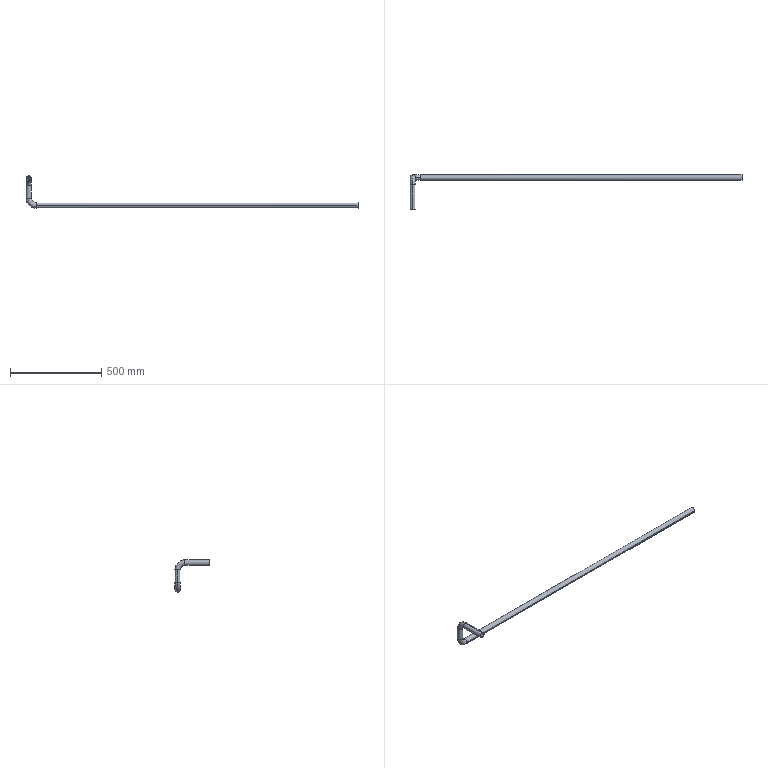Part | SolidWorks | features 3DProfileFeature 2, Sweep 1 | 1 solid | 22 faces | box 1817 x 186.765 x 176.777 mm | volume 367085 mm3 | cylinder 12 | torus 8 | plane 2 | commonest cylinder face diameters 26 x6 30 x6
STEP:
#1=CARTESIAN_POINT('',(-2187.,3372.936,-6.777));
#2=VERTEX_POINT('',#1);
#3=CARTESIAN_POINT('',(-2213.,3372.936,-6.777));
#4=VERTEX_POINT('',#3);
#5=CARTESIAN_POINT('',(-2200.,3372.936,-6.777));
#6=DIRECTION('',(0.,0.,1.));
#7=DIRECTION('',(-1.,0.,0.));
#8=AXIS2_PLACEMENT_3D('',#5,#6,#7);
#9=CIRCLE('',#8,13.);
#10=EDGE_CURVE('',#2,#4,#9,.T.);
#11=ORIENTED_EDGE('',*,*,#10,.T.);
#12=CARTESIAN_POINT('',(-2160.,3372.936,-59.777));
#13=VERTEX_POINT('',#12);
#14=CARTESIAN_POINT('',(-2160.,3372.936,-6.777));
#15=DIRECTION('',(0.,-1.,0.));
#16=DIRECTION('',(0.,0.,-1.));
#17=AXIS2_PLACEMENT_3D('',#14,#15,#16);
#18=CIRCLE('',#17,53.);
#19=EDGE_CURVE('',#4,#13,#18,.T.);
#20=ORIENTED_EDGE('',*,*,#19,.T.);
#21=CARTESIAN_POINT('',(-2160.,3385.936,-46.777));
#22=VERTEX_POINT('',#21);
#23=CARTESIAN_POINT('',(-2160.,3372.936,-46.777));
#24=DIRECTION('',(-1.,0.,0.));
#25=DIRECTION('',(0.,0.,1.));
#26=AXIS2_PLACEMENT_3D('',#23,#24,#25);
#27=CIRCLE('',#26,13.);
#28=EDGE_CURVE('',#22,#13,#27,.T.);
#29=ORIENTED_EDGE('',*,*,#28,.F.);
#30=CARTESIAN_POINT('',(-2160.,3372.936,-33.777));
#31=VERTEX_POINT('',#30);
#32=CARTESIAN_POINT('',(-2160.,3372.936,-46.777));
#33=DIRECTION('',(-1.,0.,0.));
#34=DIRECTION('',(0.,0.,1.));
#35=AXIS2_PLACEMENT_3D('',#32,#33,#34);
#36=CIRCLE('',#35,13.);
#37=EDGE_CURVE('',#31,#22,#36,.T.);
#38=ORIENTED_EDGE('',*,*,#37,.F.);
#39=CARTESIAN_POINT('',(-2160.,3372.936,-6.777));
#40=DIRECTION('',(0.,-1.,0.));
#41=DIRECTION('',(0.,0.,-1.));
#42=AXIS2_PLACEMENT_3D('',#39,#40,#41);
#43=CIRCLE('',#42,27.);
#44=EDGE_CURVE('',#2,#31,#43,.T.);
#45=ORIENTED_EDGE('',*,*,#44,.F.);
#46=EDGE_LOOP('',(#11,#20,#29,#38,#45));
#47=FACE_OUTER_BOUND('',#46,.T.);
#48=CARTESIAN_POINT('',(-2160.,3372.936,-6.777));
#49=DIRECTION('',(0.,-1.,0.));
#50=DIRECTION('',(0.,0.,-1.));
#51=AXIS2_PLACEMENT_3D('',#48,#49,#50);
#52=TOROIDAL_SURFACE('',#51,40.,13.);
#53=ADVANCED_FACE('',(#47),#52,.F.);
#54=CARTESIAN_POINT('',(-2200.,3332.936,87.));
#55=VERTEX_POINT('',#54);
#56=CARTESIAN_POINT('',(-2200.,3332.936,113.));
#57=VERTEX_POINT('',#56);
#58=CARTESIAN_POINT('',(-2200.,3332.936,100.));
#59=DIRECTION('',(0.,-1.,0.));
#60=DIRECTION('',(0.,0.,1.));
#61=AXIS2_PLACEMENT_3D('',#58,#59,#60);
#62=CIRCLE('',#61,13.);
#63=EDGE_CURVE('',#55,#57,#62,.T.);
#64=ORIENTED_EDGE('',*,*,#63,.T.);
#65=CARTESIAN_POINT('',(-2200.,3385.936,60.));
#66=VERTEX_POINT('',#65);
#67=CARTESIAN_POINT('',(-2200.,3332.936,60.));
#68=DIRECTION('',(-1.,0.,0.));
#69=DIRECTION('',(0.,0.,1.));
#70=AXIS2_PLACEMENT_3D('',#67,#68,#69);
#71=CIRCLE('',#70,53.);
#72=EDGE_CURVE('',#57,#66,#71,.T.);
#73=ORIENTED_EDGE('',*,*,#72,.T.);
#74=CARTESIAN_POINT('',(-2187.,3372.936,60.));
#75=VERTEX_POINT('',#74);
#76=CARTESIAN_POINT('',(-2200.,3372.936,60.));
#77=DIRECTION('',(0.,0.,1.));
#78=DIRECTION('',(0.,-1.,0.));
#79=AXIS2_PLACEMENT_3D('',#76,#77,#78);
#80=CIRCLE('',#79,13.);
#81=EDGE_CURVE('',#75,#66,#80,.T.);
#82=ORIENTED_EDGE('',*,*,#81,.F.);
#83=CARTESIAN_POINT('',(-2200.,3359.936,60.));
#84=VERTEX_POINT('',#83);
#85=CARTESIAN_POINT('',(-2200.,3372.936,60.));
#86=DIRECTION('',(0.,0.,1.));
#87=DIRECTION('',(0.,-1.,0.));
#88=AXIS2_PLACEMENT_3D('',#85,#86,#87);
#89=CIRCLE('',#88,13.);
#90=EDGE_CURVE('',#84,#75,#89,.T.);
#91=ORIENTED_EDGE('',*,*,#90,.F.);
#92=CARTESIAN_POINT('',(-2200.,3332.936,60.));
#93=DIRECTION('',(-1.,0.,0.));
#94=DIRECTION('',(0.,0.,1.));
#95=AXIS2_PLACEMENT_3D('',#92,#93,#94);
#96=CIRCLE('',#95,27.);
#97=EDGE_CURVE('',#55,#84,#96,.T.);
#98=ORIENTED_EDGE('',*,*,#97,.F.);
#99=EDGE_LOOP('',(#64,#73,#82,#91,#98));
#100=FACE_OUTER_BOUND('',#99,.T.);
#101=CARTESIAN_POINT('',(-2200.,3332.936,60.));
#102=DIRECTION('',(-1.,0.,0.));
#103=DIRECTION('',(0.,0.,1.));
#104=AXIS2_PLACEMENT_3D('',#101,#102,#103);
#105=TOROIDAL_SURFACE('',#104,40.,13.);
#106=ADVANCED_FACE('',(#100),#105,.F.);
#107=CARTESIAN_POINT('',(-2215.,3372.936,-6.777));
#108=VERTEX_POINT('',#107);
#109=CARTESIAN_POINT('',(-2185.,3372.936,-6.777));
#110=VERTEX_POINT('',#109);
#111=CARTESIAN_POINT('',(-2200.,3372.936,-6.777));
#112=DIRECTION('',(0.,0.,1.));
#113=DIRECTION('',(0.,-1.,0.));
#114=AXIS2_PLACEMENT_3D('',#111,#112,#113);
#115=CIRCLE('',#114,15.);
#116=EDGE_CURVE('',#108,#110,#115,.T.);
#117=ORIENTED_EDGE('',*,*,#116,.F.);
#118=CARTESIAN_POINT('',(-2160.,3372.936,-61.777));
#119=VERTEX_POINT('',#118);
#120=CARTESIAN_POINT('',(-2160.,3372.936,-6.777));
#121=DIRECTION('',(0.,-1.,0.));
#122=DIRECTION('',(0.,0.,-1.));
#123=AXIS2_PLACEMENT_3D('',#120,#121,#122);
#124=CIRCLE('',#123,55.);
#125=EDGE_CURVE('',#108,#119,#124,.T.);
#126=ORIENTED_EDGE('',*,*,#125,.T.);
#127=CARTESIAN_POINT('',(-2160.,3357.936,-46.777));
#128=VERTEX_POINT('',#127);
#129=CARTESIAN_POINT('',(-2160.,3372.936,-46.777));
#130=DIRECTION('',(-1.,0.,0.));
#131=DIRECTION('',(0.,-1.,0.));
#132=AXIS2_PLACEMENT_3D('',#129,#130,#131);
#133=CIRCLE('',#132,15.);
#134=EDGE_CURVE('',#119,#128,#133,.T.);
#135=ORIENTED_EDGE('',*,*,#134,.T.);
#136=CARTESIAN_POINT('',(-2160.,3372.936,-31.777));
#137=VERTEX_POINT('',#136);
#138=CARTESIAN_POINT('',(-2160.,3372.936,-46.777));
#139=DIRECTION('',(-1.,0.,0.));
#140=DIRECTION('',(0.,-1.,0.));
#141=AXIS2_PLACEMENT_3D('',#138,#139,#140);
#142=CIRCLE('',#141,15.);
#143=EDGE_CURVE('',#128,#137,#142,.T.);
#144=ORIENTED_EDGE('',*,*,#143,.T.);
#145=CARTESIAN_POINT('',(-2160.,3372.936,-6.777));
#146=DIRECTION('',(0.,-1.,0.));
#147=DIRECTION('',(0.,0.,-1.));
#148=AXIS2_PLACEMENT_3D('',#145,#146,#147);
#149=CIRCLE('',#148,25.);
#150=EDGE_CURVE('',#110,#137,#149,.T.);
#151=ORIENTED_EDGE('',*,*,#150,.F.);
#152=EDGE_LOOP('',(#117,#126,#135,#144,#151));
#153=FACE_OUTER_BOUND('',#152,.T.);
#154=CARTESIAN_POINT('',(-2160.,3372.936,-6.777));
#155=DIRECTION('',(0.,-1.,0.));
#156=DIRECTION('',(0.,0.,-1.));
#157=AXIS2_PLACEMENT_3D('',#154,#155,#156);
#158=TOROIDAL_SURFACE('',#157,40.,15.);
#159=ADVANCED_FACE('',(#153),#158,.T.);
#160=CARTESIAN_POINT('',(-2200.,3332.936,115.));
#161=VERTEX_POINT('',#160);
#162=CARTESIAN_POINT('',(-2200.,3332.936,85.));
#163=VERTEX_POINT('',#162);
#164=CARTESIAN_POINT('',(-2200.,3332.936,100.));
#165=DIRECTION('',(0.,-1.,0.));
#166=DIRECTION('',(0.,0.,-1.));
#167=AXIS2_PLACEMENT_3D('',#164,#165,#166);
#168=CIRCLE('',#167,15.);
#169=EDGE_CURVE('',#161,#163,#168,.T.);
#170=ORIENTED_EDGE('',*,*,#169,.F.);
#171=CARTESIAN_POINT('',(-2200.,3387.936,60.));
#172=VERTEX_POINT('',#171);
#173=CARTESIAN_POINT('',(-2200.,3332.936,60.));
#174=DIRECTION('',(-1.,0.,0.));
#175=DIRECTION('',(0.,0.,1.));
#176=AXIS2_PLACEMENT_3D('',#173,#174,#175);
#177=CIRCLE('',#176,55.);
#178=EDGE_CURVE('',#161,#172,#177,.T.);
#179=ORIENTED_EDGE('',*,*,#178,.T.);
#180=CARTESIAN_POINT('',(-2215.,3372.936,60.));
#181=VERTEX_POINT('',#180);
#182=CARTESIAN_POINT('',(-2200.,3372.936,60.));
#183=DIRECTION('',(0.,0.,1.));
#184=DIRECTION('',(0.,-1.,0.));
#185=AXIS2_PLACEMENT_3D('',#182,#183,#184);
#186=CIRCLE('',#185,15.);
#187=EDGE_CURVE('',#172,#181,#186,.T.);
#188=ORIENTED_EDGE('',*,*,#187,.T.);
#189=CARTESIAN_POINT('',(-2200.,3357.936,60.));
#190=VERTEX_POINT('',#189);
#191=CARTESIAN_POINT('',(-2200.,3372.936,60.));
#192=DIRECTION('',(0.,0.,1.));
#193=DIRECTION('',(0.,-1.,0.));
#194=AXIS2_PLACEMENT_3D('',#191,#192,#193);
#195=CIRCLE('',#194,15.);
#196=EDGE_CURVE('',#181,#190,#195,.T.);
#197=ORIENTED_EDGE('',*,*,#196,.T.);
#198=CARTESIAN_POINT('',(-2200.,3332.936,60.));
#199=DIRECTION('',(-1.,0.,0.));
#200=DIRECTION('',(0.,0.,1.));
#201=AXIS2_PLACEMENT_3D('',#198,#199,#200);
#202=CIRCLE('',#201,25.);
#203=EDGE_CURVE('',#163,#190,#202,.T.);
#204=ORIENTED_EDGE('',*,*,#203,.F.);
#205=EDGE_LOOP('',(#170,#179,#188,#197,#204));
#206=FACE_OUTER_BOUND('',#205,.T.);
#207=CARTESIAN_POINT('',(-2200.,3332.936,60.));
#208=DIRECTION('',(-1.,0.,0.));
#209=DIRECTION('',(0.,0.,1.));
#210=AXIS2_PLACEMENT_3D('',#207,#208,#209);
#211=TOROIDAL_SURFACE('',#210,40.,15.);
#212=ADVANCED_FACE('',(#206),#211,.T.);
#213=ORIENTED_EDGE('',*,*,#28,.T.);
#214=CARTESIAN_POINT('',(-2160.,3359.936,-46.777));
#215=VERTEX_POINT('',#214);
#216=CARTESIAN_POINT('',(-2160.,3372.936,-46.777));
#217=DIRECTION('',(-1.,0.,0.));
#218=DIRECTION('',(0.,0.,1.));
#219=AXIS2_PLACEMENT_3D('',#216,#217,#218);
#220=CIRCLE('',#219,13.);
#221=EDGE_CURVE('',#13,#215,#220,.T.);
#222=ORIENTED_EDGE('',*,*,#221,.T.);
#223=CARTESIAN_POINT('',(-397.658,3359.936,-46.777));
#224=VERTEX_POINT('',#223);
#225=CARTESIAN_POINT('',(-2160.,3359.936,-46.777));
#226=DIRECTION('',(1.,0.,0.));
#227=VECTOR('',#226,1000.);
#228=LINE('',#225,#227);
#229=EDGE_CURVE('',#215,#224,#228,.T.);
#230=ORIENTED_EDGE('',*,*,#229,.T.);
#231=CARTESIAN_POINT('',(-397.658,3385.936,-46.777));
#232=VERTEX_POINT('',#231);
#233=CARTESIAN_POINT('',(-397.658,3372.936,-46.777));
#234=DIRECTION('',(-1.,0.,0.));
#235=DIRECTION('',(0.,-1.,0.));
#236=AXIS2_PLACEMENT_3D('',#233,#234,#235);
#237=CIRCLE('',#236,13.);
#238=EDGE_CURVE('',#232,#224,#237,.T.);
#239=ORIENTED_EDGE('',*,*,#238,.F.);
#240=CARTESIAN_POINT('',(-2160.,3385.936,-46.777));
#241=DIRECTION('',(1.,0.,0.));
#242=VECTOR('',#241,1000.);
#243=LINE('',#240,#242);
#244=EDGE_CURVE('',#22,#232,#243,.T.);
#245=ORIENTED_EDGE('',*,*,#244,.F.);
#246=EDGE_LOOP('',(#213,#222,#230,#239,#245));
#247=FACE_OUTER_BOUND('',#246,.T.);
#248=CARTESIAN_POINT('',(-2160.,3372.936,-46.777));
#249=DIRECTION('',(1.,0.,0.));
#250=DIRECTION('',(0.,1.,0.));
#251=AXIS2_PLACEMENT_3D('',#248,#249,#250);
#252=CYLINDRICAL_SURFACE('',#251,13.);
#253=ADVANCED_FACE('',(#247),#252,.F.);
#254=CARTESIAN_POINT('',(-2213.,3372.936,60.));
#255=VERTEX_POINT('',#254);
#256=CARTESIAN_POINT('',(-2200.,3372.936,60.));
#257=DIRECTION('',(0.,0.,1.));
#258=DIRECTION('',(0.,-1.,0.));
#259=AXIS2_PLACEMENT_3D('',#256,#257,#258);
#260=CIRCLE('',#259,13.);
#261=EDGE_CURVE('',#255,#84,#260,.T.);
#262=ORIENTED_EDGE('',*,*,#261,.T.);
#263=ORIENTED_EDGE('',*,*,#90,.T.);
#264=CARTESIAN_POINT('',(-2187.,3372.936,60.));
#265=DIRECTION('',(0.,0.,-1.));
#266=VECTOR('',#265,1000.);
#267=LINE('',#264,#266);
#268=EDGE_CURVE('',#75,#2,#267,.T.);
#269=ORIENTED_EDGE('',*,*,#268,.T.);
#270=CARTESIAN_POINT('',(-2200.,3372.936,-6.777));
#271=DIRECTION('',(0.,0.,1.));
#272=DIRECTION('',(-1.,0.,0.));
#273=AXIS2_PLACEMENT_3D('',#270,#271,#272);
#274=CIRCLE('',#273,13.);
#275=EDGE_CURVE('',#4,#2,#274,.T.);
#276=ORIENTED_EDGE('',*,*,#275,.F.);
#277=CARTESIAN_POINT('',(-2213.,3372.936,60.));
#278=DIRECTION('',(0.,0.,-1.));
#279=VECTOR('',#278,1000.);
#280=LINE('',#277,#279);
#281=EDGE_CURVE('',#255,#4,#280,.T.);
#282=ORIENTED_EDGE('',*,*,#281,.F.);
#283=EDGE_LOOP('',(#262,#263,#269,#276,#282));
#284=FACE_OUTER_BOUND('',#283,.T.);
#285=CARTESIAN_POINT('',(-2200.,3372.936,60.));
#286=DIRECTION('',(0.,0.,-1.));
#287=DIRECTION('',(-1.,0.,0.));
#288=AXIS2_PLACEMENT_3D('',#285,#286,#287);
#289=CYLINDRICAL_SURFACE('',#288,13.);
#290=ADVANCED_FACE('',(#284),#289,.F.);
#291=CARTESIAN_POINT('',(-2200.,3201.171,113.));
#292=VERTEX_POINT('',#291);
#293=CARTESIAN_POINT('',(-2200.,3201.171,87.));
#294=VERTEX_POINT('',#293);
#295=CARTESIAN_POINT('',(-2200.,3201.171,100.));
#296=DIRECTION('',(0.,-1.,0.));
#297=DIRECTION('',(0.,0.,-1.));
#298=AXIS2_PLACEMENT_3D('',#295,#296,#297);
#299=CIRCLE('',#298,13.);
#300=EDGE_CURVE('',#292,#294,#299,.T.);
#301=ORIENTED_EDGE('',*,*,#300,.T.);
#302=CARTESIAN_POINT('',(-2200.,3201.171,87.));
#303=DIRECTION('',(0.,1.,0.));
#304=VECTOR('',#303,1000.);
#305=LINE('',#302,#304);
#306=EDGE_CURVE('',#294,#55,#305,.T.);
#307=ORIENTED_EDGE('',*,*,#306,.T.);
#308=CARTESIAN_POINT('',(-2200.,3332.936,100.));
#309=DIRECTION('',(0.,-1.,0.));
#310=DIRECTION('',(0.,0.,1.));
#311=AXIS2_PLACEMENT_3D('',#308,#309,#310);
#312=CIRCLE('',#311,13.);
#313=EDGE_CURVE('',#57,#55,#312,.T.);
#314=ORIENTED_EDGE('',*,*,#313,.F.);
#315=CARTESIAN_POINT('',(-2200.,3201.171,113.));
#316=DIRECTION('',(0.,1.,0.));
#317=VECTOR('',#316,1000.);
#318=LINE('',#315,#317);
#319=EDGE_CURVE('',#292,#57,#318,.T.);
#320=ORIENTED_EDGE('',*,*,#319,.F.);
#321=EDGE_LOOP('',(#301,#307,#314,#320));
#322=FACE_OUTER_BOUND('',#321,.T.);
#323=CARTESIAN_POINT('',(-2200.,3201.171,100.));
#324=DIRECTION('',(0.,1.,0.));
#325=DIRECTION('',(0.,0.,1.));
#326=AXIS2_PLACEMENT_3D('',#323,#324,#325);
#327=CYLINDRICAL_SURFACE('',#326,13.);
#328=ADVANCED_FACE('',(#322),#327,.F.);
#329=ORIENTED_EDGE('',*,*,#143,.F.);
#330=CARTESIAN_POINT('',(-397.658,3357.936,-46.777));
#331=VERTEX_POINT('',#330);
#332=CARTESIAN_POINT('',(-2160.,3357.936,-46.777));
#333=DIRECTION('',(1.,0.,0.));
#334=VECTOR('',#333,1000.);
#335=LINE('',#332,#334);
#336=EDGE_CURVE('',#128,#331,#335,.T.);
#337=ORIENTED_EDGE('',*,*,#336,.T.);
#338=CARTESIAN_POINT('',(-397.658,3387.936,-46.777));
#339=VERTEX_POINT('',#338);
#340=CARTESIAN_POINT('',(-397.658,3372.936,-46.777));
#341=DIRECTION('',(-1.,0.,0.));
#342=DIRECTION('',(0.,-1.,0.));
#343=AXIS2_PLACEMENT_3D('',#340,#341,#342);
#344=CIRCLE('',#343,15.);
#345=EDGE_CURVE('',#331,#339,#344,.T.);
#346=ORIENTED_EDGE('',*,*,#345,.T.);
#347=CARTESIAN_POINT('',(-2160.,3387.936,-46.777));
#348=VERTEX_POINT('',#347);
#349=CARTESIAN_POINT('',(-2160.,3387.936,-46.777));
#350=DIRECTION('',(1.,0.,0.));
#351=VECTOR('',#350,1000.);
#352=LINE('',#349,#351);
#353=EDGE_CURVE('',#348,#339,#352,.T.);
#354=ORIENTED_EDGE('',*,*,#353,.F.);
#355=CARTESIAN_POINT('',(-2160.,3372.936,-46.777));
#356=DIRECTION('',(-1.,0.,0.));
#357=DIRECTION('',(0.,-1.,0.));
#358=AXIS2_PLACEMENT_3D('',#355,#356,#357);
#359=CIRCLE('',#358,15.);
#360=EDGE_CURVE('',#137,#348,#359,.T.);
#361=ORIENTED_EDGE('',*,*,#360,.F.);
#362=EDGE_LOOP('',(#329,#337,#346,#354,#361));
#363=FACE_OUTER_BOUND('',#362,.T.);
#364=CARTESIAN_POINT('',(-2160.,3372.936,-46.777));
#365=DIRECTION('',(1.,0.,0.));
#366=DIRECTION('',(0.,1.,0.));
#367=AXIS2_PLACEMENT_3D('',#364,#365,#366);
#368=CYLINDRICAL_SURFACE('',#367,15.);
#369=ADVANCED_FACE('',(#363),#368,.T.);
#370=CARTESIAN_POINT('',(-2185.,3372.936,60.));
#371=VERTEX_POINT('',#370);
#372=CARTESIAN_POINT('',(-2200.,3372.936,60.));
#373=DIRECTION('',(0.,0.,1.));
#374=DIRECTION('',(0.,-1.,0.));
#375=AXIS2_PLACEMENT_3D('',#372,#373,#374);
#376=CIRCLE('',#375,15.);
#377=EDGE_CURVE('',#371,#172,#376,.T.);
#378=ORIENTED_EDGE('',*,*,#377,.F.);
#379=CARTESIAN_POINT('',(-2185.,3372.936,60.));
#380=DIRECTION('',(0.,0.,-1.));
#381=VECTOR('',#380,1000.);
#382=LINE('',#379,#381);
#383=EDGE_CURVE('',#371,#110,#382,.T.);
#384=ORIENTED_EDGE('',*,*,#383,.T.);
#385=CARTESIAN_POINT('',(-2200.,3372.936,-6.777));
#386=DIRECTION('',(0.,0.,1.));
#387=DIRECTION('',(0.,-1.,0.));
#388=AXIS2_PLACEMENT_3D('',#385,#386,#387);
#389=CIRCLE('',#388,15.);
#390=EDGE_CURVE('',#110,#108,#389,.T.);
#391=ORIENTED_EDGE('',*,*,#390,.T.);
#392=CARTESIAN_POINT('',(-2215.,3372.936,60.));
#393=DIRECTION('',(0.,0.,-1.));
#394=VECTOR('',#393,1000.);
#395=LINE('',#392,#394);
#396=EDGE_CURVE('',#181,#108,#395,.T.);
#397=ORIENTED_EDGE('',*,*,#396,.F.);
#398=ORIENTED_EDGE('',*,*,#187,.F.);
#399=EDGE_LOOP('',(#378,#384,#391,#397,#398));
#400=FACE_OUTER_BOUND('',#399,.T.);
#401=CARTESIAN_POINT('',(-2200.,3372.936,60.));
#402=DIRECTION('',(0.,0.,-1.));
#403=DIRECTION('',(-1.,0.,0.));
#404=AXIS2_PLACEMENT_3D('',#401,#402,#403);
#405=CYLINDRICAL_SURFACE('',#404,15.);
#406=ADVANCED_FACE('',(#400),#405,.T.);
#407=CARTESIAN_POINT('',(-2200.,3201.171,85.));
#408=VERTEX_POINT('',#407);
#409=CARTESIAN_POINT('',(-2200.,3201.171,115.));
#410=VERTEX_POINT('',#409);
#411=CARTESIAN_POINT('',(-2200.,3201.171,100.));
#412=DIRECTION('',(0.,-1.,0.));
#413=DIRECTION('',(0.,0.,-1.));
#414=AXIS2_PLACEMENT_3D('',#411,#412,#413);
#415=CIRCLE('',#414,15.);
#416=EDGE_CURVE('',#408,#410,#415,.T.);
#417=ORIENTED_EDGE('',*,*,#416,.F.);
#418=CARTESIAN_POINT('',(-2200.,3201.171,85.));
#419=DIRECTION('',(0.,1.,0.));
#420=VECTOR('',#419,1000.);
#421=LINE('',#418,#420);
#422=EDGE_CURVE('',#408,#163,#421,.T.);
#423=ORIENTED_EDGE('',*,*,#422,.T.);
#424=CARTESIAN_POINT('',(-2200.,3332.936,100.));
#425=DIRECTION('',(0.,-1.,0.));
#426=DIRECTION('',(0.,0.,-1.));
#427=AXIS2_PLACEMENT_3D('',#424,#425,#426);
#428=CIRCLE('',#427,15.);
#429=EDGE_CURVE('',#163,#161,#428,.T.);
#430=ORIENTED_EDGE('',*,*,#429,.T.);
#431=CARTESIAN_POINT('',(-2200.,3201.171,115.));
#432=DIRECTION('',(0.,1.,0.));
#433=VECTOR('',#432,1000.);
#434=LINE('',#431,#433);
#435=EDGE_CURVE('',#410,#161,#434,.T.);
#436=ORIENTED_EDGE('',*,*,#435,.F.);
#437=EDGE_LOOP('',(#417,#423,#430,#436));
#438=FACE_OUTER_BOUND('',#437,.T.);
#439=CARTESIAN_POINT('',(-2200.,3201.171,100.));
#440=DIRECTION('',(0.,1.,0.));
#441=DIRECTION('',(0.,0.,1.));
#442=AXIS2_PLACEMENT_3D('',#439,#440,#441);
#443=CYLINDRICAL_SURFACE('',#442,15.);
#444=ADVANCED_FACE('',(#438),#443,.T.);
#445=ORIENTED_EDGE('',*,*,#336,.F.);
#446=ORIENTED_EDGE('',*,*,#134,.F.);
#447=CARTESIAN_POINT('',(-2160.,3372.936,-46.777));
#448=DIRECTION('',(-1.,0.,0.));
#449=DIRECTION('',(0.,-1.,0.));
#450=AXIS2_PLACEMENT_3D('',#447,#448,#449);
#451=CIRCLE('',#450,15.);
#452=EDGE_CURVE('',#348,#119,#451,.T.);
#453=ORIENTED_EDGE('',*,*,#452,.F.);
#454=ORIENTED_EDGE('',*,*,#353,.T.);
#455=CARTESIAN_POINT('',(-397.658,3372.936,-46.777));
#456=DIRECTION('',(-1.,0.,0.));
#457=DIRECTION('',(0.,-1.,0.));
#458=AXIS2_PLACEMENT_3D('',#455,#456,#457);
#459=CIRCLE('',#458,15.);
#460=EDGE_CURVE('',#339,#331,#459,.T.);
#461=ORIENTED_EDGE('',*,*,#460,.T.);
#462=EDGE_LOOP('',(#445,#446,#453,#454,#461));
#463=FACE_OUTER_BOUND('',#462,.T.);
#464=CARTESIAN_POINT('',(-2160.,3372.936,-46.777));
#465=DIRECTION('',(1.,0.,0.));
#466=DIRECTION('',(0.,1.,0.));
#467=AXIS2_PLACEMENT_3D('',#464,#465,#466);
#468=CYLINDRICAL_SURFACE('',#467,15.);
#469=ADVANCED_FACE('',(#463),#468,.T.);
#470=ORIENTED_EDGE('',*,*,#125,.F.);
#471=ORIENTED_EDGE('',*,*,#390,.F.);
#472=ORIENTED_EDGE('',*,*,#150,.T.);
#473=ORIENTED_EDGE('',*,*,#360,.T.);
#474=ORIENTED_EDGE('',*,*,#452,.T.);
#475=EDGE_LOOP('',(#470,#471,#472,#473,#474));
#476=FACE_OUTER_BOUND('',#475,.T.);
#477=CARTESIAN_POINT('',(-2160.,3372.936,-6.777));
#478=DIRECTION('',(0.,-1.,0.));
#479=DIRECTION('',(0.,0.,-1.));
#480=AXIS2_PLACEMENT_3D('',#477,#478,#479);
#481=TOROIDAL_SURFACE('',#480,40.,15.);
#482=ADVANCED_FACE('',(#476),#481,.T.);
#483=ORIENTED_EDGE('',*,*,#383,.F.);
#484=CARTESIAN_POINT('',(-2200.,3372.936,60.));
#485=DIRECTION('',(0.,0.,1.));
#486=DIRECTION('',(0.,-1.,0.));
#487=AXIS2_PLACEMENT_3D('',#484,#485,#486);
#488=CIRCLE('',#487,15.);
#489=EDGE_CURVE('',#190,#371,#488,.T.);
#490=ORIENTED_EDGE('',*,*,#489,.F.);
#491=ORIENTED_EDGE('',*,*,#196,.F.);
#492=ORIENTED_EDGE('',*,*,#396,.T.);
#493=ORIENTED_EDGE('',*,*,#116,.T.);
#494=EDGE_LOOP('',(#483,#490,#491,#492,#493));
#495=FACE_OUTER_BOUND('',#494,.T.);
#496=CARTESIAN_POINT('',(-2200.,3372.936,60.));
#497=DIRECTION('',(0.,0.,-1.));
#498=DIRECTION('',(-1.,0.,0.));
#499=AXIS2_PLACEMENT_3D('',#496,#497,#498);
#500=CYLINDRICAL_SURFACE('',#499,15.);
#501=ADVANCED_FACE('',(#495),#500,.T.);
#502=ORIENTED_EDGE('',*,*,#178,.F.);
#503=ORIENTED_EDGE('',*,*,#429,.F.);
#504=ORIENTED_EDGE('',*,*,#203,.T.);
#505=ORIENTED_EDGE('',*,*,#489,.T.);
#506=ORIENTED_EDGE('',*,*,#377,.T.);
#507=EDGE_LOOP('',(#502,#503,#504,#505,#506));
#508=FACE_OUTER_BOUND('',#507,.T.);
#509=CARTESIAN_POINT('',(-2200.,3332.936,60.));
#510=DIRECTION('',(-1.,0.,0.));
#511=DIRECTION('',(0.,0.,1.));
#512=AXIS2_PLACEMENT_3D('',#509,#510,#511);
#513=TOROIDAL_SURFACE('',#512,40.,15.);
#514=ADVANCED_FACE('',(#508),#513,.T.);
#515=ORIENTED_EDGE('',*,*,#422,.F.);
#516=CARTESIAN_POINT('',(-2200.,3201.171,100.));
#517=DIRECTION('',(0.,-1.,0.));
#518=DIRECTION('',(0.,0.,-1.));
#519=AXIS2_PLACEMENT_3D('',#516,#517,#518);
#520=CIRCLE('',#519,15.);
#521=EDGE_CURVE('',#410,#408,#520,.T.);
#522=ORIENTED_EDGE('',*,*,#521,.F.);
#523=ORIENTED_EDGE('',*,*,#435,.T.);
#524=ORIENTED_EDGE('',*,*,#169,.T.);
#525=EDGE_LOOP('',(#515,#522,#523,#524));
#526=FACE_OUTER_BOUND('',#525,.T.);
#527=CARTESIAN_POINT('',(-2200.,3201.171,100.));
#528=DIRECTION('',(0.,1.,0.));
#529=DIRECTION('',(0.,0.,1.));
#530=AXIS2_PLACEMENT_3D('',#527,#528,#529);
#531=CYLINDRICAL_SURFACE('',#530,15.);
#532=ADVANCED_FACE('',(#526),#531,.T.);
#533=ORIENTED_EDGE('',*,*,#238,.T.);
#534=CARTESIAN_POINT('',(-397.658,3372.936,-46.777));
#535=DIRECTION('',(-1.,0.,0.));
#536=DIRECTION('',(0.,-1.,0.));
#537=AXIS2_PLACEMENT_3D('',#534,#535,#536);
#538=CIRCLE('',#537,13.);
#539=EDGE_CURVE('',#224,#232,#538,.T.);
#540=ORIENTED_EDGE('',*,*,#539,.T.);
#541=EDGE_LOOP('',(#533,#540));
#542=FACE_BOUND('',#541,.T.);
#543=ORIENTED_EDGE('',*,*,#460,.F.);
#544=ORIENTED_EDGE('',*,*,#345,.F.);
#545=EDGE_LOOP('',(#543,#544));
#546=FACE_OUTER_BOUND('',#545,.T.);
#547=CARTESIAN_POINT('',(-397.658,3372.936,-46.777));
#548=DIRECTION('',(-1.,0.,0.));
#549=DIRECTION('',(0.,-1.,0.));
#550=AXIS2_PLACEMENT_3D('',#547,#548,#549);
#551=PLANE('',#550);
#552=ADVANCED_FACE('',(#542,#546),#551,.F.);
#553=ORIENTED_EDGE('',*,*,#300,.F.);
#554=CARTESIAN_POINT('',(-2200.,3201.171,100.));
#555=DIRECTION('',(0.,-1.,0.));
#556=DIRECTION('',(0.,0.,-1.));
#557=AXIS2_PLACEMENT_3D('',#554,#555,#556);
#558=CIRCLE('',#557,13.);
#559=EDGE_CURVE('',#294,#292,#558,.T.);
#560=ORIENTED_EDGE('',*,*,#559,.F.);
#561=EDGE_LOOP('',(#553,#560));
#562=FACE_BOUND('',#561,.T.);
#563=ORIENTED_EDGE('',*,*,#521,.T.);
#564=ORIENTED_EDGE('',*,*,#416,.T.);
#565=EDGE_LOOP('',(#563,#564));
#566=FACE_OUTER_BOUND('',#565,.T.);
#567=CARTESIAN_POINT('',(-2200.,3201.171,100.));
#568=DIRECTION('',(0.,-1.,0.));
#569=DIRECTION('',(0.,0.,-1.));
#570=AXIS2_PLACEMENT_3D('',#567,#568,#569);
#571=PLANE('',#570);
#572=ADVANCED_FACE('',(#562,#566),#571,.T.);
#573=ORIENTED_EDGE('',*,*,#229,.F.);
#574=CARTESIAN_POINT('',(-2160.,3372.936,-46.777));
#575=DIRECTION('',(-1.,0.,0.));
#576=DIRECTION('',(0.,0.,1.));
#577=AXIS2_PLACEMENT_3D('',#574,#575,#576);
#578=CIRCLE('',#577,13.);
#579=EDGE_CURVE('',#215,#31,#578,.T.);
#580=ORIENTED_EDGE('',*,*,#579,.T.);
#581=ORIENTED_EDGE('',*,*,#37,.T.);
#582=ORIENTED_EDGE('',*,*,#244,.T.);
#583=ORIENTED_EDGE('',*,*,#539,.F.);
#584=EDGE_LOOP('',(#573,#580,#581,#582,#583));
#585=FACE_OUTER_BOUND('',#584,.T.);
#586=CARTESIAN_POINT('',(-2160.,3372.936,-46.777));
#587=DIRECTION('',(1.,0.,0.));
#588=DIRECTION('',(0.,1.,0.));
#589=AXIS2_PLACEMENT_3D('',#586,#587,#588);
#590=CYLINDRICAL_SURFACE('',#589,13.);
#591=ADVANCED_FACE('',(#585),#590,.F.);
#592=ORIENTED_EDGE('',*,*,#19,.F.);
#593=ORIENTED_EDGE('',*,*,#275,.T.);
#594=ORIENTED_EDGE('',*,*,#44,.T.);
#595=ORIENTED_EDGE('',*,*,#579,.F.);
#596=ORIENTED_EDGE('',*,*,#221,.F.);
#597=EDGE_LOOP('',(#592,#593,#594,#595,#596));
#598=FACE_OUTER_BOUND('',#597,.T.);
#599=CARTESIAN_POINT('',(-2160.,3372.936,-6.777));
#600=DIRECTION('',(0.,-1.,0.));
#601=DIRECTION('',(0.,0.,-1.));
#602=AXIS2_PLACEMENT_3D('',#599,#600,#601);
#603=TOROIDAL_SURFACE('',#602,40.,13.);
#604=ADVANCED_FACE('',(#598),#603,.F.);
#605=ORIENTED_EDGE('',*,*,#268,.F.);
#606=ORIENTED_EDGE('',*,*,#81,.T.);
#607=CARTESIAN_POINT('',(-2200.,3372.936,60.));
#608=DIRECTION('',(0.,0.,1.));
#609=DIRECTION('',(0.,-1.,0.));
#610=AXIS2_PLACEMENT_3D('',#607,#608,#609);
#611=CIRCLE('',#610,13.);
#612=EDGE_CURVE('',#66,#255,#611,.T.);
#613=ORIENTED_EDGE('',*,*,#612,.T.);
#614=ORIENTED_EDGE('',*,*,#281,.T.);
#615=ORIENTED_EDGE('',*,*,#10,.F.);
#616=EDGE_LOOP('',(#605,#606,#613,#614,#615));
#617=FACE_OUTER_BOUND('',#616,.T.);
#618=CARTESIAN_POINT('',(-2200.,3372.936,60.));
#619=DIRECTION('',(0.,0.,-1.));
#620=DIRECTION('',(-1.,0.,0.));
#621=AXIS2_PLACEMENT_3D('',#618,#619,#620);
#622=CYLINDRICAL_SURFACE('',#621,13.);
#623=ADVANCED_FACE('',(#617),#622,.F.);
#624=ORIENTED_EDGE('',*,*,#72,.F.);
#625=ORIENTED_EDGE('',*,*,#313,.T.);
#626=ORIENTED_EDGE('',*,*,#97,.T.);
#627=ORIENTED_EDGE('',*,*,#261,.F.);
#628=ORIENTED_EDGE('',*,*,#612,.F.);
#629=EDGE_LOOP('',(#624,#625,#626,#627,#628));
#630=FACE_OUTER_BOUND('',#629,.T.);
#631=CARTESIAN_POINT('',(-2200.,3332.936,60.));
#632=DIRECTION('',(-1.,0.,0.));
#633=DIRECTION('',(0.,0.,1.));
#634=AXIS2_PLACEMENT_3D('',#631,#632,#633);
#635=TOROIDAL_SURFACE('',#634,40.,13.);
#636=ADVANCED_FACE('',(#630),#635,.F.);
#637=ORIENTED_EDGE('',*,*,#306,.F.);
#638=ORIENTED_EDGE('',*,*,#559,.T.);
#639=ORIENTED_EDGE('',*,*,#319,.T.);
#640=ORIENTED_EDGE('',*,*,#63,.F.);
#641=EDGE_LOOP('',(#637,#638,#639,#640));
#642=FACE_OUTER_BOUND('',#641,.T.);
#643=CARTESIAN_POINT('',(-2200.,3201.171,100.));
#644=DIRECTION('',(0.,1.,0.));
#645=DIRECTION('',(0.,0.,1.));
#646=AXIS2_PLACEMENT_3D('',#643,#644,#645);
#647=CYLINDRICAL_SURFACE('',#646,13.);
#648=ADVANCED_FACE('',(#642),#647,.F.);
#649=CLOSED_SHELL('',(#53,#106,#159,#212,#253,#290,#328,#369,#406,#444,#469,#482,#501,#514,#532,#552,#572,#591,#604,#623,#636,#648));
#650=MANIFOLD_SOLID_BREP('',#649);
#651=CARTESIAN_POINT('',(0.,0.,0.));
#652=DIRECTION('',(0.,0.,1.));
#653=DIRECTION('',(1.,0.,0.));
#654=AXIS2_PLACEMENT_3D('',#651,#652,#653);
#655=(LENGTH_UNIT()NAMED_UNIT(*)SI_UNIT(.MILLI.,.METRE.));
#656=UNCERTAINTY_MEASURE_WITH_UNIT(LENGTH_MEASURE(0.00001),#655,'','');
#657=(NAMED_UNIT(*)PLANE_ANGLE_UNIT()SI_UNIT($,.RADIAN.));
#658=(NAMED_UNIT(*)SI_UNIT($,.STERADIAN.)SOLID_ANGLE_UNIT());
#659=(GEOMETRIC_REPRESENTATION_CONTEXT(3)GLOBAL_UNCERTAINTY_ASSIGNED_CONTEXT((#656))GLOBAL_UNIT_ASSIGNED_CONTEXT((#655,#657,#658))REPRESENTATION_CONTEXT('',''));
#660=ADVANCED_BREP_SHAPE_REPRESENTATION('',(#650,#654),#659);